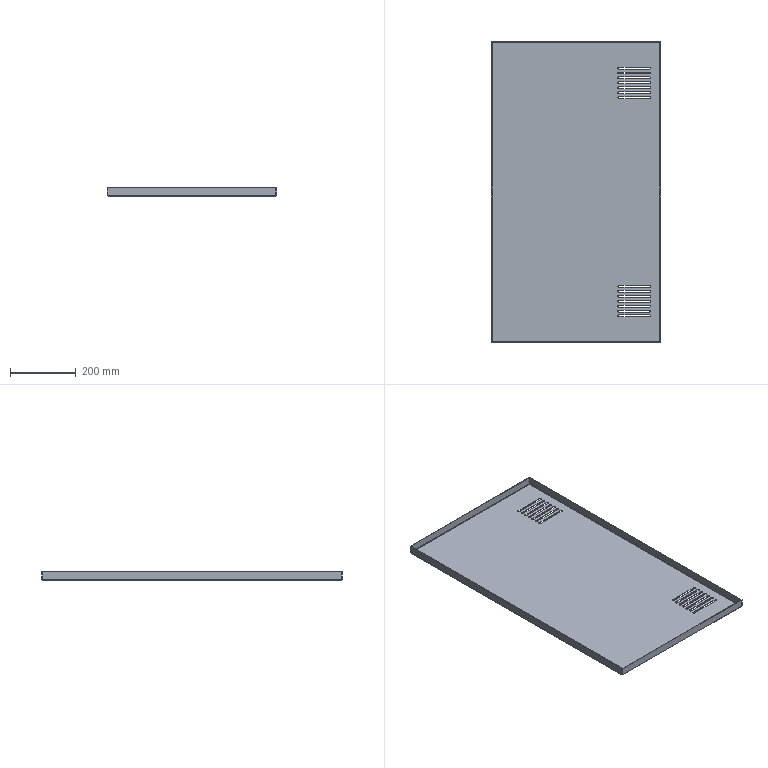Part | STEP file | SynoNew-0304-052 | 1 solid | 98 faces | box 515 x 915 x 25 mm | volume 790603 mm3 | plane 62 | cylinder 36 | commonest cylinder face diameters 6 x32 3 x4